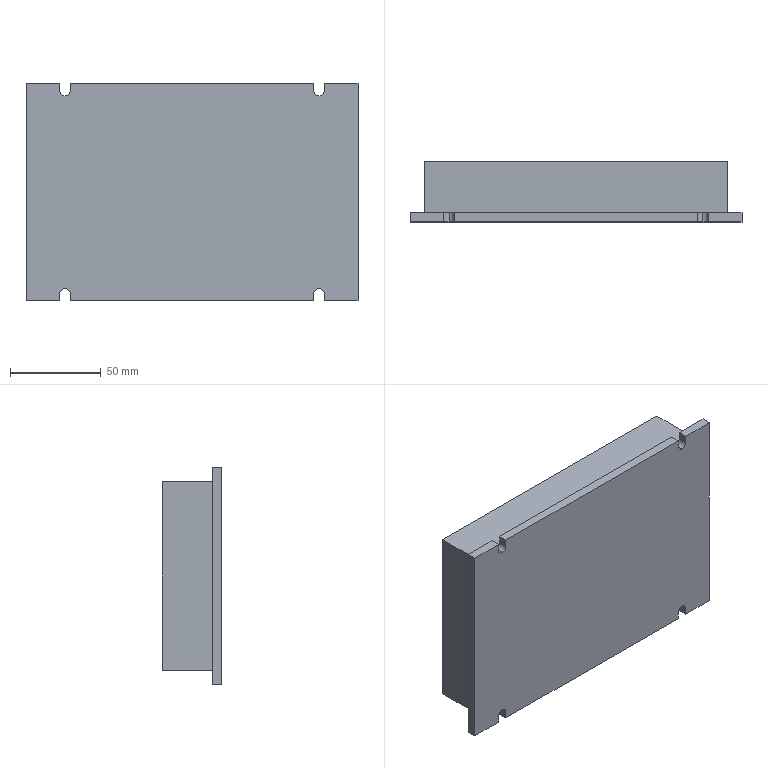Part | SolidWorks | features Extrusion 1, HoleWzd 1, ICE 1 | 1 solid | 29 faces | box 183 x 33 x 120 mm | volume 595376 mm3 | plane 23 | cylinder 6 | commonest cylinder face diameters 5.8 x6
STEP:
#1=CARTESIAN_POINT('',(-70.,5.,53.1));
#2=VERTEX_POINT('',#1);
#3=CARTESIAN_POINT('',(-67.1,5.,56.));
#4=VERTEX_POINT('',#3);
#5=CARTESIAN_POINT('',(-70.,5.,56.));
#6=DIRECTION('',(0.,-1.,0.));
#7=DIRECTION('',(0.,0.,-1.));
#8=AXIS2_PLACEMENT_3D('',#5,#6,#7);
#9=CIRCLE('',#8,2.9);
#10=EDGE_CURVE('',#2,#4,#9,.T.);
#11=ORIENTED_EDGE('',*,*,#10,.F.);
#12=CARTESIAN_POINT('',(-70.,0.,53.1));
#13=VERTEX_POINT('',#12);
#14=CARTESIAN_POINT('',(-70.,0.,53.1));
#15=DIRECTION('',(0.,-1.,0.));
#16=VECTOR('',#15,1000.);
#17=LINE('',#14,#16);
#18=EDGE_CURVE('',#2,#13,#17,.T.);
#19=ORIENTED_EDGE('',*,*,#18,.T.);
#20=CARTESIAN_POINT('',(-67.1,0.,56.));
#21=VERTEX_POINT('',#20);
#22=CARTESIAN_POINT('',(-70.,0.,56.));
#23=DIRECTION('',(0.,-1.,0.));
#24=DIRECTION('',(0.,0.,-1.));
#25=AXIS2_PLACEMENT_3D('',#22,#23,#24);
#26=CIRCLE('',#25,2.9);
#27=EDGE_CURVE('',#13,#21,#26,.T.);
#28=ORIENTED_EDGE('',*,*,#27,.T.);
#29=CARTESIAN_POINT('',(-67.1,33.,56.));
#30=DIRECTION('',(0.,1.,0.));
#31=VECTOR('',#30,1000.);
#32=LINE('',#29,#31);
#33=EDGE_CURVE('',#21,#4,#32,.T.);
#34=ORIENTED_EDGE('',*,*,#33,.T.);
#35=EDGE_LOOP('',(#11,#19,#28,#34));
#36=FACE_OUTER_BOUND('',#35,.T.);
#37=CARTESIAN_POINT('',(-70.,0.,56.));
#38=DIRECTION('',(0.,-1.,0.));
#39=DIRECTION('',(0.,0.,-1.));
#40=AXIS2_PLACEMENT_3D('',#37,#38,#39);
#41=CYLINDRICAL_SURFACE('',#40,2.9);
#42=ADVANCED_FACE('',(#36),#41,.F.);
#43=CARTESIAN_POINT('',(70.,5.,53.1));
#44=VERTEX_POINT('',#43);
#45=CARTESIAN_POINT('',(72.9,5.,56.));
#46=VERTEX_POINT('',#45);
#47=CARTESIAN_POINT('',(70.,5.,56.));
#48=DIRECTION('',(0.,-1.,0.));
#49=DIRECTION('',(0.,0.,-1.));
#50=AXIS2_PLACEMENT_3D('',#47,#48,#49);
#51=CIRCLE('',#50,2.9);
#52=EDGE_CURVE('',#44,#46,#51,.T.);
#53=ORIENTED_EDGE('',*,*,#52,.F.);
#54=CARTESIAN_POINT('',(70.,0.,53.1));
#55=VERTEX_POINT('',#54);
#56=CARTESIAN_POINT('',(70.,0.,53.1));
#57=DIRECTION('',(0.,-1.,0.));
#58=VECTOR('',#57,1000.);
#59=LINE('',#56,#58);
#60=EDGE_CURVE('',#44,#55,#59,.T.);
#61=ORIENTED_EDGE('',*,*,#60,.T.);
#62=CARTESIAN_POINT('',(72.9,0.,56.));
#63=VERTEX_POINT('',#62);
#64=CARTESIAN_POINT('',(70.,0.,56.));
#65=DIRECTION('',(0.,-1.,0.));
#66=DIRECTION('',(0.,0.,-1.));
#67=AXIS2_PLACEMENT_3D('',#64,#65,#66);
#68=CIRCLE('',#67,2.9);
#69=EDGE_CURVE('',#55,#63,#68,.T.);
#70=ORIENTED_EDGE('',*,*,#69,.T.);
#71=CARTESIAN_POINT('',(72.9,33.,56.));
#72=DIRECTION('',(0.,1.,0.));
#73=VECTOR('',#72,1000.);
#74=LINE('',#71,#73);
#75=EDGE_CURVE('',#63,#46,#74,.T.);
#76=ORIENTED_EDGE('',*,*,#75,.T.);
#77=EDGE_LOOP('',(#53,#61,#70,#76));
#78=FACE_OUTER_BOUND('',#77,.T.);
#79=CARTESIAN_POINT('',(70.,0.,56.));
#80=DIRECTION('',(0.,-1.,0.));
#81=DIRECTION('',(0.,0.,-1.));
#82=AXIS2_PLACEMENT_3D('',#79,#80,#81);
#83=CYLINDRICAL_SURFACE('',#82,2.9);
#84=ADVANCED_FACE('',(#78),#83,.F.);
#85=CARTESIAN_POINT('',(-83.5,5.,52.));
#86=VERTEX_POINT('',#85);
#87=CARTESIAN_POINT('',(83.5,5.,52.));
#88=VERTEX_POINT('',#87);
#89=CARTESIAN_POINT('',(-83.5,5.,52.));
#90=DIRECTION('',(1.,0.,0.));
#91=VECTOR('',#90,1000.);
#92=LINE('',#89,#91);
#93=EDGE_CURVE('',#86,#88,#92,.T.);
#94=ORIENTED_EDGE('',*,*,#93,.F.);
#95=CARTESIAN_POINT('',(-83.5,5.,-52.));
#96=VERTEX_POINT('',#95);
#97=CARTESIAN_POINT('',(-83.5,5.,-52.));
#98=DIRECTION('',(0.,0.,1.));
#99=VECTOR('',#98,1000.);
#100=LINE('',#97,#99);
#101=EDGE_CURVE('',#96,#86,#100,.T.);
#102=ORIENTED_EDGE('',*,*,#101,.F.);
#103=CARTESIAN_POINT('',(83.5,5.,-52.));
#104=VERTEX_POINT('',#103);
#105=CARTESIAN_POINT('',(83.5,5.,-52.));
#106=DIRECTION('',(-1.,0.,0.));
#107=VECTOR('',#106,1000.);
#108=LINE('',#105,#107);
#109=EDGE_CURVE('',#104,#96,#108,.T.);
#110=ORIENTED_EDGE('',*,*,#109,.F.);
#111=CARTESIAN_POINT('',(83.5,5.,52.));
#112=DIRECTION('',(0.,0.,-1.));
#113=VECTOR('',#112,1000.);
#114=LINE('',#111,#113);
#115=EDGE_CURVE('',#88,#104,#114,.T.);
#116=ORIENTED_EDGE('',*,*,#115,.F.);
#117=EDGE_LOOP('',(#94,#102,#110,#116));
#118=FACE_BOUND('',#117,.T.);
#119=CARTESIAN_POINT('',(72.9,5.,-56.));
#120=VERTEX_POINT('',#119);
#121=CARTESIAN_POINT('',(72.9,5.,-60.));
#122=VERTEX_POINT('',#121);
#123=CARTESIAN_POINT('',(72.9,5.,0.));
#124=DIRECTION('',(0.,0.,-1.));
#125=VECTOR('',#124,1000.);
#126=LINE('',#123,#125);
#127=EDGE_CURVE('',#120,#122,#126,.T.);
#128=ORIENTED_EDGE('',*,*,#127,.F.);
#129=CARTESIAN_POINT('',(67.1,5.,-56.));
#130=VERTEX_POINT('',#129);
#131=CARTESIAN_POINT('',(70.,5.,-56.));
#132=DIRECTION('',(0.,-1.,0.));
#133=DIRECTION('',(0.,0.,-1.));
#134=AXIS2_PLACEMENT_3D('',#131,#132,#133);
#135=CIRCLE('',#134,2.9);
#136=EDGE_CURVE('',#120,#130,#135,.T.);
#137=ORIENTED_EDGE('',*,*,#136,.T.);
#138=CARTESIAN_POINT('',(67.1,5.,-60.));
#139=VERTEX_POINT('',#138);
#140=CARTESIAN_POINT('',(67.1,5.,0.));
#141=DIRECTION('',(0.,0.,-1.));
#142=VECTOR('',#141,1000.);
#143=LINE('',#140,#142);
#144=EDGE_CURVE('',#130,#139,#143,.T.);
#145=ORIENTED_EDGE('',*,*,#144,.T.);
#146=CARTESIAN_POINT('',(-67.1,5.,-60.));
#147=VERTEX_POINT('',#146);
#148=CARTESIAN_POINT('',(-91.5,5.,-60.));
#149=DIRECTION('',(-1.,0.,0.));
#150=VECTOR('',#149,1000.);
#151=LINE('',#148,#150);
#152=EDGE_CURVE('',#139,#147,#151,.T.);
#153=ORIENTED_EDGE('',*,*,#152,.T.);
#154=CARTESIAN_POINT('',(-67.1,5.,-56.));
#155=VERTEX_POINT('',#154);
#156=CARTESIAN_POINT('',(-67.1,5.,0.));
#157=DIRECTION('',(0.,0.,-1.));
#158=VECTOR('',#157,1000.);
#159=LINE('',#156,#158);
#160=EDGE_CURVE('',#155,#147,#159,.T.);
#161=ORIENTED_EDGE('',*,*,#160,.F.);
#162=CARTESIAN_POINT('',(-72.9,5.,-56.));
#163=VERTEX_POINT('',#162);
#164=CARTESIAN_POINT('',(-70.,5.,-56.));
#165=DIRECTION('',(0.,-1.,0.));
#166=DIRECTION('',(0.,0.,-1.));
#167=AXIS2_PLACEMENT_3D('',#164,#165,#166);
#168=CIRCLE('',#167,2.9);
#169=EDGE_CURVE('',#155,#163,#168,.T.);
#170=ORIENTED_EDGE('',*,*,#169,.T.);
#171=CARTESIAN_POINT('',(-72.9,5.,-60.));
#172=VERTEX_POINT('',#171);
#173=CARTESIAN_POINT('',(-72.9,5.,0.));
#174=DIRECTION('',(0.,0.,-1.));
#175=VECTOR('',#174,1000.);
#176=LINE('',#173,#175);
#177=EDGE_CURVE('',#163,#172,#176,.T.);
#178=ORIENTED_EDGE('',*,*,#177,.T.);
#179=CARTESIAN_POINT('',(-91.5,5.,-60.));
#180=VERTEX_POINT('',#179);
#181=CARTESIAN_POINT('',(-91.5,5.,-60.));
#182=DIRECTION('',(-1.,0.,0.));
#183=VECTOR('',#182,1000.);
#184=LINE('',#181,#183);
#185=EDGE_CURVE('',#172,#180,#184,.T.);
#186=ORIENTED_EDGE('',*,*,#185,.T.);
#187=CARTESIAN_POINT('',(-91.5,5.,60.));
#188=VERTEX_POINT('',#187);
#189=CARTESIAN_POINT('',(-91.5,5.,60.));
#190=DIRECTION('',(0.,0.,1.));
#191=VECTOR('',#190,1000.);
#192=LINE('',#189,#191);
#193=EDGE_CURVE('',#180,#188,#192,.T.);
#194=ORIENTED_EDGE('',*,*,#193,.T.);
#195=CARTESIAN_POINT('',(-72.9,5.,60.));
#196=VERTEX_POINT('',#195);
#197=CARTESIAN_POINT('',(-91.5,5.,60.));
#198=DIRECTION('',(1.,0.,0.));
#199=VECTOR('',#198,1000.);
#200=LINE('',#197,#199);
#201=EDGE_CURVE('',#188,#196,#200,.T.);
#202=ORIENTED_EDGE('',*,*,#201,.T.);
#203=CARTESIAN_POINT('',(-72.9,5.,56.));
#204=VERTEX_POINT('',#203);
#205=CARTESIAN_POINT('',(-72.9,5.,0.));
#206=DIRECTION('',(0.,0.,-1.));
#207=VECTOR('',#206,1000.);
#208=LINE('',#205,#207);
#209=EDGE_CURVE('',#196,#204,#208,.T.);
#210=ORIENTED_EDGE('',*,*,#209,.T.);
#211=CARTESIAN_POINT('',(-70.,5.,56.));
#212=DIRECTION('',(0.,-1.,0.));
#213=DIRECTION('',(0.,0.,-1.));
#214=AXIS2_PLACEMENT_3D('',#211,#212,#213);
#215=CIRCLE('',#214,2.9);
#216=EDGE_CURVE('',#204,#2,#215,.T.);
#217=ORIENTED_EDGE('',*,*,#216,.T.);
#218=ORIENTED_EDGE('',*,*,#10,.T.);
#219=CARTESIAN_POINT('',(-67.1,5.,60.));
#220=VERTEX_POINT('',#219);
#221=CARTESIAN_POINT('',(-67.1,5.,0.));
#222=DIRECTION('',(0.,0.,-1.));
#223=VECTOR('',#222,1000.);
#224=LINE('',#221,#223);
#225=EDGE_CURVE('',#220,#4,#224,.T.);
#226=ORIENTED_EDGE('',*,*,#225,.F.);
#227=CARTESIAN_POINT('',(67.1,5.,60.));
#228=VERTEX_POINT('',#227);
#229=CARTESIAN_POINT('',(-91.5,5.,60.));
#230=DIRECTION('',(1.,0.,0.));
#231=VECTOR('',#230,1000.);
#232=LINE('',#229,#231);
#233=EDGE_CURVE('',#220,#228,#232,.T.);
#234=ORIENTED_EDGE('',*,*,#233,.T.);
#235=CARTESIAN_POINT('',(67.1,5.,56.));
#236=VERTEX_POINT('',#235);
#237=CARTESIAN_POINT('',(67.1,5.,0.));
#238=DIRECTION('',(0.,0.,-1.));
#239=VECTOR('',#238,1000.);
#240=LINE('',#237,#239);
#241=EDGE_CURVE('',#228,#236,#240,.T.);
#242=ORIENTED_EDGE('',*,*,#241,.T.);
#243=CARTESIAN_POINT('',(70.,5.,56.));
#244=DIRECTION('',(0.,-1.,0.));
#245=DIRECTION('',(0.,0.,-1.));
#246=AXIS2_PLACEMENT_3D('',#243,#244,#245);
#247=CIRCLE('',#246,2.9);
#248=EDGE_CURVE('',#236,#44,#247,.T.);
#249=ORIENTED_EDGE('',*,*,#248,.T.);
#250=ORIENTED_EDGE('',*,*,#52,.T.);
#251=CARTESIAN_POINT('',(72.9,5.,60.));
#252=VERTEX_POINT('',#251);
#253=CARTESIAN_POINT('',(72.9,5.,0.));
#254=DIRECTION('',(0.,0.,-1.));
#255=VECTOR('',#254,1000.);
#256=LINE('',#253,#255);
#257=EDGE_CURVE('',#252,#46,#256,.T.);
#258=ORIENTED_EDGE('',*,*,#257,.F.);
#259=CARTESIAN_POINT('',(91.5,5.,60.));
#260=VERTEX_POINT('',#259);
#261=CARTESIAN_POINT('',(-91.5,5.,60.));
#262=DIRECTION('',(1.,0.,0.));
#263=VECTOR('',#262,1000.);
#264=LINE('',#261,#263);
#265=EDGE_CURVE('',#252,#260,#264,.T.);
#266=ORIENTED_EDGE('',*,*,#265,.T.);
#267=CARTESIAN_POINT('',(91.5,5.,-60.));
#268=VERTEX_POINT('',#267);
#269=CARTESIAN_POINT('',(91.5,5.,60.));
#270=DIRECTION('',(0.,0.,-1.));
#271=VECTOR('',#270,1000.);
#272=LINE('',#269,#271);
#273=EDGE_CURVE('',#260,#268,#272,.T.);
#274=ORIENTED_EDGE('',*,*,#273,.T.);
#275=CARTESIAN_POINT('',(-91.5,5.,-60.));
#276=DIRECTION('',(-1.,0.,0.));
#277=VECTOR('',#276,1000.);
#278=LINE('',#275,#277);
#279=EDGE_CURVE('',#268,#122,#278,.T.);
#280=ORIENTED_EDGE('',*,*,#279,.T.);
#281=EDGE_LOOP('',(#128,#137,#145,#153,#161,#170,#178,#186,#194,#202,#210,#217,#218,#226,#234,#242,#249,#250,#258,#266,#274,#280));
#282=FACE_OUTER_BOUND('',#281,.T.);
#283=CARTESIAN_POINT('',(0.,5.,0.));
#284=DIRECTION('',(0.,-1.,0.));
#285=DIRECTION('',(0.,0.,-1.));
#286=AXIS2_PLACEMENT_3D('',#283,#284,#285);
#287=PLANE('',#286);
#288=ADVANCED_FACE('',(#118,#282),#287,.F.);
#289=CARTESIAN_POINT('',(72.9,0.,-60.));
#290=VERTEX_POINT('',#289);
#291=CARTESIAN_POINT('',(72.9,5.,-60.));
#292=DIRECTION('',(0.,-1.,0.));
#293=VECTOR('',#292,1000.);
#294=LINE('',#291,#293);
#295=EDGE_CURVE('',#122,#290,#294,.T.);
#296=ORIENTED_EDGE('',*,*,#295,.F.);
#297=ORIENTED_EDGE('',*,*,#279,.F.);
#298=CARTESIAN_POINT('',(91.5,0.,-60.));
#299=VERTEX_POINT('',#298);
#300=CARTESIAN_POINT('',(91.5,5.,-60.));
#301=DIRECTION('',(0.,-1.,0.));
#302=VECTOR('',#301,1000.);
#303=LINE('',#300,#302);
#304=EDGE_CURVE('',#268,#299,#303,.T.);
#305=ORIENTED_EDGE('',*,*,#304,.T.);
#306=CARTESIAN_POINT('',(-91.5,0.,-60.));
#307=DIRECTION('',(-1.,0.,0.));
#308=VECTOR('',#307,1000.);
#309=LINE('',#306,#308);
#310=EDGE_CURVE('',#299,#290,#309,.T.);
#311=ORIENTED_EDGE('',*,*,#310,.T.);
#312=EDGE_LOOP('',(#296,#297,#305,#311));
#313=FACE_OUTER_BOUND('',#312,.T.);
#314=CARTESIAN_POINT('',(-91.5,5.,-60.));
#315=DIRECTION('',(0.,0.,1.));
#316=DIRECTION('',(1.,0.,0.));
#317=AXIS2_PLACEMENT_3D('',#314,#315,#316);
#318=PLANE('',#317);
#319=ADVANCED_FACE('',(#313),#318,.F.);
#320=CARTESIAN_POINT('',(72.9,0.,-56.));
#321=VERTEX_POINT('',#320);
#322=CARTESIAN_POINT('',(67.1,0.,-56.));
#323=VERTEX_POINT('',#322);
#324=CARTESIAN_POINT('',(70.,0.,-56.));
#325=DIRECTION('',(0.,-1.,0.));
#326=DIRECTION('',(0.,0.,-1.));
#327=AXIS2_PLACEMENT_3D('',#324,#325,#326);
#328=CIRCLE('',#327,2.9);
#329=EDGE_CURVE('',#321,#323,#328,.T.);
#330=ORIENTED_EDGE('',*,*,#329,.F.);
#331=CARTESIAN_POINT('',(72.9,0.,-56.));
#332=DIRECTION('',(0.,0.,-1.));
#333=VECTOR('',#332,1000.);
#334=LINE('',#331,#333);
#335=EDGE_CURVE('',#321,#290,#334,.T.);
#336=ORIENTED_EDGE('',*,*,#335,.T.);
#337=ORIENTED_EDGE('',*,*,#310,.F.);
#338=CARTESIAN_POINT('',(91.5,0.,60.));
#339=VERTEX_POINT('',#338);
#340=CARTESIAN_POINT('',(91.5,0.,60.));
#341=DIRECTION('',(0.,0.,-1.));
#342=VECTOR('',#341,1000.);
#343=LINE('',#340,#342);
#344=EDGE_CURVE('',#339,#299,#343,.T.);
#345=ORIENTED_EDGE('',*,*,#344,.F.);
#346=CARTESIAN_POINT('',(72.9,0.,60.));
#347=VERTEX_POINT('',#346);
#348=CARTESIAN_POINT('',(-91.5,0.,60.));
#349=DIRECTION('',(1.,0.,0.));
#350=VECTOR('',#349,1000.);
#351=LINE('',#348,#350);
#352=EDGE_CURVE('',#347,#339,#351,.T.);
#353=ORIENTED_EDGE('',*,*,#352,.F.);
#354=CARTESIAN_POINT('',(72.9,0.,64.));
#355=DIRECTION('',(0.,0.,-1.));
#356=VECTOR('',#355,1000.);
#357=LINE('',#354,#356);
#358=EDGE_CURVE('',#347,#63,#357,.T.);
#359=ORIENTED_EDGE('',*,*,#358,.T.);
#360=ORIENTED_EDGE('',*,*,#69,.F.);
#361=CARTESIAN_POINT('',(67.1,0.,56.));
#362=VERTEX_POINT('',#361);
#363=CARTESIAN_POINT('',(70.,0.,56.));
#364=DIRECTION('',(0.,-1.,0.));
#365=DIRECTION('',(0.,0.,-1.));
#366=AXIS2_PLACEMENT_3D('',#363,#364,#365);
#367=CIRCLE('',#366,2.9);
#368=EDGE_CURVE('',#362,#55,#367,.T.);
#369=ORIENTED_EDGE('',*,*,#368,.F.);
#370=CARTESIAN_POINT('',(67.1,0.,60.));
#371=VERTEX_POINT('',#370);
#372=CARTESIAN_POINT('',(67.1,0.,0.));
#373=DIRECTION('',(0.,0.,-1.));
#374=VECTOR('',#373,1000.);
#375=LINE('',#372,#374);
#376=EDGE_CURVE('',#371,#362,#375,.T.);
#377=ORIENTED_EDGE('',*,*,#376,.F.);
#378=CARTESIAN_POINT('',(-67.1,0.,60.));
#379=VERTEX_POINT('',#378);
#380=CARTESIAN_POINT('',(-91.5,0.,60.));
#381=DIRECTION('',(1.,0.,0.));
#382=VECTOR('',#381,1000.);
#383=LINE('',#380,#382);
#384=EDGE_CURVE('',#379,#371,#383,.T.);
#385=ORIENTED_EDGE('',*,*,#384,.F.);
#386=CARTESIAN_POINT('',(-67.1,0.,64.));
#387=DIRECTION('',(0.,0.,-1.));
#388=VECTOR('',#387,1000.);
#389=LINE('',#386,#388);
#390=EDGE_CURVE('',#379,#21,#389,.T.);
#391=ORIENTED_EDGE('',*,*,#390,.T.);
#392=ORIENTED_EDGE('',*,*,#27,.F.);
#393=CARTESIAN_POINT('',(-72.9,0.,56.));
#394=VERTEX_POINT('',#393);
#395=CARTESIAN_POINT('',(-70.,0.,56.));
#396=DIRECTION('',(0.,-1.,0.));
#397=DIRECTION('',(0.,0.,-1.));
#398=AXIS2_PLACEMENT_3D('',#395,#396,#397);
#399=CIRCLE('',#398,2.9);
#400=EDGE_CURVE('',#394,#13,#399,.T.);
#401=ORIENTED_EDGE('',*,*,#400,.F.);
#402=CARTESIAN_POINT('',(-72.9,0.,60.));
#403=VERTEX_POINT('',#402);
#404=CARTESIAN_POINT('',(-72.9,0.,64.));
#405=DIRECTION('',(0.,0.,-1.));
#406=VECTOR('',#405,1000.);
#407=LINE('',#404,#406);
#408=EDGE_CURVE('',#403,#394,#407,.T.);
#409=ORIENTED_EDGE('',*,*,#408,.F.);
#410=CARTESIAN_POINT('',(-91.5,0.,60.));
#411=VERTEX_POINT('',#410);
#412=CARTESIAN_POINT('',(-91.5,0.,60.));
#413=DIRECTION('',(1.,0.,0.));
#414=VECTOR('',#413,1000.);
#415=LINE('',#412,#414);
#416=EDGE_CURVE('',#411,#403,#415,.T.);
#417=ORIENTED_EDGE('',*,*,#416,.F.);
#418=CARTESIAN_POINT('',(-91.5,0.,-60.));
#419=VERTEX_POINT('',#418);
#420=CARTESIAN_POINT('',(-91.5,0.,60.));
#421=DIRECTION('',(0.,0.,1.));
#422=VECTOR('',#421,1000.);
#423=LINE('',#420,#422);
#424=EDGE_CURVE('',#419,#411,#423,.T.);
#425=ORIENTED_EDGE('',*,*,#424,.F.);
#426=CARTESIAN_POINT('',(-72.9,0.,-60.));
#427=VERTEX_POINT('',#426);
#428=CARTESIAN_POINT('',(-91.5,0.,-60.));
#429=DIRECTION('',(-1.,0.,0.));
#430=VECTOR('',#429,1000.);
#431=LINE('',#428,#430);
#432=EDGE_CURVE('',#427,#419,#431,.T.);
#433=ORIENTED_EDGE('',*,*,#432,.F.);
#434=CARTESIAN_POINT('',(-72.9,0.,-56.));
#435=VERTEX_POINT('',#434);
#436=CARTESIAN_POINT('',(-72.9,0.,-56.));
#437=DIRECTION('',(0.,0.,-1.));
#438=VECTOR('',#437,1000.);
#439=LINE('',#436,#438);
#440=EDGE_CURVE('',#435,#427,#439,.T.);
#441=ORIENTED_EDGE('',*,*,#440,.F.);
#442=CARTESIAN_POINT('',(-67.1,0.,-56.));
#443=VERTEX_POINT('',#442);
#444=CARTESIAN_POINT('',(-70.,0.,-56.));
#445=DIRECTION('',(0.,-1.,0.));
#446=DIRECTION('',(0.,0.,-1.));
#447=AXIS2_PLACEMENT_3D('',#444,#445,#446);
#448=CIRCLE('',#447,2.9);
#449=EDGE_CURVE('',#443,#435,#448,.T.);
#450=ORIENTED_EDGE('',*,*,#449,.F.);
#451=CARTESIAN_POINT('',(-67.1,0.,-60.));
#452=VERTEX_POINT('',#451);
#453=CARTESIAN_POINT('',(-67.1,0.,-56.));
#454=DIRECTION('',(0.,0.,-1.));
#455=VECTOR('',#454,1000.);
#456=LINE('',#453,#455);
#457=EDGE_CURVE('',#443,#452,#456,.T.);
#458=ORIENTED_EDGE('',*,*,#457,.T.);
#459=CARTESIAN_POINT('',(67.1,0.,-60.));
#460=VERTEX_POINT('',#459);
#461=CARTESIAN_POINT('',(-91.5,0.,-60.));
#462=DIRECTION('',(-1.,0.,0.));
#463=VECTOR('',#462,1000.);
#464=LINE('',#461,#463);
#465=EDGE_CURVE('',#460,#452,#464,.T.);
#466=ORIENTED_EDGE('',*,*,#465,.F.);
#467=CARTESIAN_POINT('',(67.1,0.,-56.));
#468=DIRECTION('',(0.,0.,-1.));
#469=VECTOR('',#468,1000.);
#470=LINE('',#467,#469);
#471=EDGE_CURVE('',#323,#460,#470,.T.);
#472=ORIENTED_EDGE('',*,*,#471,.F.);
#473=EDGE_LOOP('',(#330,#336,#337,#345,#353,#359,#360,#369,#377,#385,#391,#392,#401,#409,#417,#425,#433,#441,#450,#458,#466,#472));
#474=FACE_OUTER_BOUND('',#473,.T.);
#475=CARTESIAN_POINT('',(0.,0.,0.));
#476=DIRECTION('',(0.,-1.,0.));
#477=DIRECTION('',(0.,0.,-1.));
#478=AXIS2_PLACEMENT_3D('',#475,#476,#477);
#479=PLANE('',#478);
#480=ADVANCED_FACE('',(#474),#479,.T.);
#481=ORIENTED_EDGE('',*,*,#152,.F.);
#482=CARTESIAN_POINT('',(67.1,5.,-60.));
#483=DIRECTION('',(0.,-1.,0.));
#484=VECTOR('',#483,1000.);
#485=LINE('',#482,#484);
#486=EDGE_CURVE('',#139,#460,#485,.T.);
#487=ORIENTED_EDGE('',*,*,#486,.T.);
#488=ORIENTED_EDGE('',*,*,#465,.T.);
#489=CARTESIAN_POINT('',(-67.1,5.,-60.));
#490=DIRECTION('',(0.,-1.,0.));
#491=VECTOR('',#490,1000.);
#492=LINE('',#489,#491);
#493=EDGE_CURVE('',#147,#452,#492,.T.);
#494=ORIENTED_EDGE('',*,*,#493,.F.);
#495=EDGE_LOOP('',(#481,#487,#488,#494));
#496=FACE_OUTER_BOUND('',#495,.T.);
#497=CARTESIAN_POINT('',(-91.5,5.,-60.));
#498=DIRECTION('',(0.,0.,1.));
#499=DIRECTION('',(1.,0.,0.));
#500=AXIS2_PLACEMENT_3D('',#497,#498,#499);
#501=PLANE('',#500);
#502=ADVANCED_FACE('',(#496),#501,.F.);
#503=CARTESIAN_POINT('',(-67.1,5.,60.));
#504=DIRECTION('',(0.,1.,0.));
#505=VECTOR('',#504,1000.);
#506=LINE('',#503,#505);
#507=EDGE_CURVE('',#379,#220,#506,.T.);
#508=ORIENTED_EDGE('',*,*,#507,.F.);
#509=ORIENTED_EDGE('',*,*,#384,.T.);
#510=CARTESIAN_POINT('',(67.1,5.,60.));
#511=DIRECTION('',(0.,1.,0.));
#512=VECTOR('',#511,1000.);
#513=LINE('',#510,#512);
#514=EDGE_CURVE('',#371,#228,#513,.T.);
#515=ORIENTED_EDGE('',*,*,#514,.T.);
#516=ORIENTED_EDGE('',*,*,#233,.F.);
#517=EDGE_LOOP('',(#508,#509,#515,#516));
#518=FACE_OUTER_BOUND('',#517,.T.);
#519=CARTESIAN_POINT('',(-91.5,5.,60.));
#520=DIRECTION('',(0.,0.,-1.));
#521=DIRECTION('',(-1.,0.,0.));
#522=AXIS2_PLACEMENT_3D('',#519,#520,#521);
#523=PLANE('',#522);
#524=ADVANCED_FACE('',(#518),#523,.F.);
#525=CARTESIAN_POINT('',(72.9,5.,60.));
#526=DIRECTION('',(0.,1.,0.));
#527=VECTOR('',#526,1000.);
#528=LINE('',#525,#527);
#529=EDGE_CURVE('',#347,#252,#528,.T.);
#530=ORIENTED_EDGE('',*,*,#529,.F.);
#531=ORIENTED_EDGE('',*,*,#352,.T.);
#532=CARTESIAN_POINT('',(91.5,5.,60.));
#533=DIRECTION('',(0.,-1.,0.));
#534=VECTOR('',#533,1000.);
#535=LINE('',#532,#534);
#536=EDGE_CURVE('',#260,#339,#535,.T.);
#537=ORIENTED_EDGE('',*,*,#536,.F.);
#538=ORIENTED_EDGE('',*,*,#265,.F.);
#539=EDGE_LOOP('',(#530,#531,#537,#538));
#540=FACE_OUTER_BOUND('',#539,.T.);
#541=CARTESIAN_POINT('',(-91.5,5.,60.));
#542=DIRECTION('',(0.,0.,-1.));
#543=DIRECTION('',(-1.,0.,0.));
#544=AXIS2_PLACEMENT_3D('',#541,#542,#543);
#545=PLANE('',#544);
#546=ADVANCED_FACE('',(#540),#545,.F.);
#547=ORIENTED_EDGE('',*,*,#344,.T.);
#548=ORIENTED_EDGE('',*,*,#304,.F.);
#549=ORIENTED_EDGE('',*,*,#273,.F.);
#550=ORIENTED_EDGE('',*,*,#536,.T.);
#551=EDGE_LOOP('',(#547,#548,#549,#550));
#552=FACE_OUTER_BOUND('',#551,.T.);
#553=CARTESIAN_POINT('',(91.5,5.,60.));
#554=DIRECTION('',(-1.,0.,0.));
#555=DIRECTION('',(0.,0.,1.));
#556=AXIS2_PLACEMENT_3D('',#553,#554,#555);
#557=PLANE('',#556);
#558=ADVANCED_FACE('',(#552),#557,.F.);
#559=ORIENTED_EDGE('',*,*,#185,.F.);
#560=CARTESIAN_POINT('',(-72.9,5.,-60.));
#561=DIRECTION('',(0.,-1.,0.));
#562=VECTOR('',#561,1000.);
#563=LINE('',#560,#562);
#564=EDGE_CURVE('',#172,#427,#563,.T.);
#565=ORIENTED_EDGE('',*,*,#564,.T.);
#566=ORIENTED_EDGE('',*,*,#432,.T.);
#567=CARTESIAN_POINT('',(-91.5,5.,-60.));
#568=DIRECTION('',(0.,-1.,0.));
#569=VECTOR('',#568,1000.);
#570=LINE('',#567,#569);
#571=EDGE_CURVE('',#180,#419,#570,.T.);
#572=ORIENTED_EDGE('',*,*,#571,.F.);
#573=EDGE_LOOP('',(#559,#565,#566,#572));
#574=FACE_OUTER_BOUND('',#573,.T.);
#575=CARTESIAN_POINT('',(-91.5,5.,-60.));
#576=DIRECTION('',(0.,0.,1.));
#577=DIRECTION('',(1.,0.,0.));
#578=AXIS2_PLACEMENT_3D('',#575,#576,#577);
#579=PLANE('',#578);
#580=ADVANCED_FACE('',(#574),#579,.F.);
#581=ORIENTED_EDGE('',*,*,#424,.T.);
#582=CARTESIAN_POINT('',(-91.5,5.,60.));
#583=DIRECTION('',(0.,-1.,0.));
#584=VECTOR('',#583,1000.);
#585=LINE('',#582,#584);
#586=EDGE_CURVE('',#188,#411,#585,.T.);
#587=ORIENTED_EDGE('',*,*,#586,.F.);
#588=ORIENTED_EDGE('',*,*,#193,.F.);
#589=ORIENTED_EDGE('',*,*,#571,.T.);
#590=EDGE_LOOP('',(#581,#587,#588,#589));
#591=FACE_OUTER_BOUND('',#590,.T.);
#592=CARTESIAN_POINT('',(-91.5,5.,60.));
#593=DIRECTION('',(1.,0.,0.));
#594=DIRECTION('',(0.,0.,-1.));
#595=AXIS2_PLACEMENT_3D('',#592,#593,#594);
#596=PLANE('',#595);
#597=ADVANCED_FACE('',(#591),#596,.F.);
#598=ORIENTED_EDGE('',*,*,#416,.T.);
#599=CARTESIAN_POINT('',(-72.9,5.,60.));
#600=DIRECTION('',(0.,1.,0.));
#601=VECTOR('',#600,1000.);
#602=LINE('',#599,#601);
#603=EDGE_CURVE('',#403,#196,#602,.T.);
#604=ORIENTED_EDGE('',*,*,#603,.T.);
#605=ORIENTED_EDGE('',*,*,#201,.F.);
#606=ORIENTED_EDGE('',*,*,#586,.T.);
#607=EDGE_LOOP('',(#598,#604,#605,#606));
#608=FACE_OUTER_BOUND('',#607,.T.);
#609=CARTESIAN_POINT('',(-91.5,5.,60.));
#610=DIRECTION('',(0.,0.,-1.));
#611=DIRECTION('',(-1.,0.,0.));
#612=AXIS2_PLACEMENT_3D('',#609,#610,#611);
#613=PLANE('',#612);
#614=ADVANCED_FACE('',(#608),#613,.F.);
#615=ORIENTED_EDGE('',*,*,#93,.T.);
#616=CARTESIAN_POINT('',(83.5,33.,52.));
#617=VERTEX_POINT('',#616);
#618=CARTESIAN_POINT('',(83.5,33.,52.));
#619=DIRECTION('',(0.,-1.,0.));
#620=VECTOR('',#619,1000.);
#621=LINE('',#618,#620);
#622=EDGE_CURVE('',#617,#88,#621,.T.);
#623=ORIENTED_EDGE('',*,*,#622,.F.);
#624=CARTESIAN_POINT('',(-83.5,33.,52.));
#625=VERTEX_POINT('',#624);
#626=CARTESIAN_POINT('',(-83.5,33.,52.));
#627=DIRECTION('',(1.,0.,0.));
#628=VECTOR('',#627,1000.);
#629=LINE('',#626,#628);
#630=EDGE_CURVE('',#625,#617,#629,.T.);
#631=ORIENTED_EDGE('',*,*,#630,.F.);
#632=CARTESIAN_POINT('',(-83.5,33.,52.));
#633=DIRECTION('',(0.,-1.,0.));
#634=VECTOR('',#633,1000.);
#635=LINE('',#632,#634);
#636=EDGE_CURVE('',#625,#86,#635,.T.);
#637=ORIENTED_EDGE('',*,*,#636,.T.);
#638=EDGE_LOOP('',(#615,#623,#631,#637));
#639=FACE_OUTER_BOUND('',#638,.T.);
#640=CARTESIAN_POINT('',(-83.5,33.,52.));
#641=DIRECTION('',(0.,0.,-1.));
#642=DIRECTION('',(-1.,0.,0.));
#643=AXIS2_PLACEMENT_3D('',#640,#641,#642);
#644=PLANE('',#643);
#645=ADVANCED_FACE('',(#639),#644,.F.);
#646=ORIENTED_EDGE('',*,*,#115,.T.);
#647=CARTESIAN_POINT('',(83.5,33.,-52.));
#648=VERTEX_POINT('',#647);
#649=CARTESIAN_POINT('',(83.5,33.,-52.));
#650=DIRECTION('',(0.,-1.,0.));
#651=VECTOR('',#650,1000.);
#652=LINE('',#649,#651);
#653=EDGE_CURVE('',#648,#104,#652,.T.);
#654=ORIENTED_EDGE('',*,*,#653,.F.);
#655=CARTESIAN_POINT('',(83.5,33.,52.));
#656=DIRECTION('',(0.,0.,-1.));
#657=VECTOR('',#656,1000.);
#658=LINE('',#655,#657);
#659=EDGE_CURVE('',#617,#648,#658,.T.);
#660=ORIENTED_EDGE('',*,*,#659,.F.);
#661=ORIENTED_EDGE('',*,*,#622,.T.);
#662=EDGE_LOOP('',(#646,#654,#660,#661));
#663=FACE_OUTER_BOUND('',#662,.T.);
#664=CARTESIAN_POINT('',(83.5,33.,52.));
#665=DIRECTION('',(-1.,0.,0.));
#666=DIRECTION('',(0.,0.,1.));
#667=AXIS2_PLACEMENT_3D('',#664,#665,#666);
#668=PLANE('',#667);
#669=ADVANCED_FACE('',(#663),#668,.F.);
#670=ORIENTED_EDGE('',*,*,#109,.T.);
#671=CARTESIAN_POINT('',(-83.5,33.,-52.));
#672=VERTEX_POINT('',#671);
#673=CARTESIAN_POINT('',(-83.5,33.,-52.));
#674=DIRECTION('',(0.,-1.,0.));
#675=VECTOR('',#674,1000.);
#676=LINE('',#673,#675);
#677=EDGE_CURVE('',#672,#96,#676,.T.);
#678=ORIENTED_EDGE('',*,*,#677,.F.);
#679=CARTESIAN_POINT('',(83.5,33.,-52.));
#680=DIRECTION('',(-1.,0.,0.));
#681=VECTOR('',#680,1000.);
#682=LINE('',#679,#681);
#683=EDGE_CURVE('',#648,#672,#682,.T.);
#684=ORIENTED_EDGE('',*,*,#683,.F.);
#685=ORIENTED_EDGE('',*,*,#653,.T.);
#686=EDGE_LOOP('',(#670,#678,#684,#685));
#687=FACE_OUTER_BOUND('',#686,.T.);
#688=CARTESIAN_POINT('',(83.5,33.,-52.));
#689=DIRECTION('',(0.,0.,1.));
#690=DIRECTION('',(1.,0.,0.));
#691=AXIS2_PLACEMENT_3D('',#688,#689,#690);
#692=PLANE('',#691);
#693=ADVANCED_FACE('',(#687),#692,.F.);
#694=ORIENTED_EDGE('',*,*,#101,.T.);
#695=ORIENTED_EDGE('',*,*,#636,.F.);
#696=CARTESIAN_POINT('',(-83.5,33.,-52.));
#697=DIRECTION('',(0.,0.,1.));
#698=VECTOR('',#697,1000.);
#699=LINE('',#696,#698);
#700=EDGE_CURVE('',#672,#625,#699,.T.);
#701=ORIENTED_EDGE('',*,*,#700,.F.);
#702=ORIENTED_EDGE('',*,*,#677,.T.);
#703=EDGE_LOOP('',(#694,#695,#701,#702));
#704=FACE_OUTER_BOUND('',#703,.T.);
#705=CARTESIAN_POINT('',(-83.5,33.,-52.));
#706=DIRECTION('',(1.,0.,0.));
#707=DIRECTION('',(0.,0.,-1.));
#708=AXIS2_PLACEMENT_3D('',#705,#706,#707);
#709=PLANE('',#708);
#710=ADVANCED_FACE('',(#704),#709,.F.);
#711=ORIENTED_EDGE('',*,*,#630,.T.);
#712=ORIENTED_EDGE('',*,*,#659,.T.);
#713=ORIENTED_EDGE('',*,*,#683,.T.);
#714=ORIENTED_EDGE('',*,*,#700,.T.);
#715=EDGE_LOOP('',(#711,#712,#713,#714));
#716=FACE_OUTER_BOUND('',#715,.T.);
#717=CARTESIAN_POINT('',(0.,33.,0.));
#718=DIRECTION('',(0.,1.,0.));
#719=DIRECTION('',(0.,0.,1.));
#720=AXIS2_PLACEMENT_3D('',#717,#718,#719);
#721=PLANE('',#720);
#722=ADVANCED_FACE('',(#716),#721,.T.);
#723=ORIENTED_EDGE('',*,*,#60,.F.);
#724=ORIENTED_EDGE('',*,*,#248,.F.);
#725=CARTESIAN_POINT('',(67.1,0.,56.));
#726=DIRECTION('',(0.,1.,0.));
#727=VECTOR('',#726,1000.);
#728=LINE('',#725,#727);
#729=EDGE_CURVE('',#362,#236,#728,.T.);
#730=ORIENTED_EDGE('',*,*,#729,.F.);
#731=ORIENTED_EDGE('',*,*,#368,.T.);
#732=EDGE_LOOP('',(#723,#724,#730,#731));
#733=FACE_OUTER_BOUND('',#732,.T.);
#734=CARTESIAN_POINT('',(70.,0.,56.));
#735=DIRECTION('',(0.,-1.,0.));
#736=DIRECTION('',(0.,0.,-1.));
#737=AXIS2_PLACEMENT_3D('',#734,#735,#736);
#738=CYLINDRICAL_SURFACE('',#737,2.9);
#739=ADVANCED_FACE('',(#733),#738,.F.);
#740=ORIENTED_EDGE('',*,*,#257,.T.);
#741=ORIENTED_EDGE('',*,*,#75,.F.);
#742=ORIENTED_EDGE('',*,*,#358,.F.);
#743=ORIENTED_EDGE('',*,*,#529,.T.);
#744=EDGE_LOOP('',(#740,#741,#742,#743));
#745=FACE_OUTER_BOUND('',#744,.T.);
#746=CARTESIAN_POINT('',(72.9,33.,64.));
#747=DIRECTION('',(-1.,0.,0.));
#748=DIRECTION('',(0.,-1.,0.));
#749=AXIS2_PLACEMENT_3D('',#746,#747,#748);
#750=PLANE('',#749);
#751=ADVANCED_FACE('',(#745),#750,.T.);
#752=ORIENTED_EDGE('',*,*,#514,.F.);
#753=ORIENTED_EDGE('',*,*,#376,.T.);
#754=ORIENTED_EDGE('',*,*,#729,.T.);
#755=ORIENTED_EDGE('',*,*,#241,.F.);
#756=EDGE_LOOP('',(#752,#753,#754,#755));
#757=FACE_OUTER_BOUND('',#756,.T.);
#758=CARTESIAN_POINT('',(67.1,0.,64.));
#759=DIRECTION('',(-1.,0.,0.));
#760=DIRECTION('',(0.,0.,1.));
#761=AXIS2_PLACEMENT_3D('',#758,#759,#760);
#762=PLANE('',#761);
#763=ADVANCED_FACE('',(#757),#762,.F.);
#764=ORIENTED_EDGE('',*,*,#18,.F.);
#765=ORIENTED_EDGE('',*,*,#216,.F.);
#766=CARTESIAN_POINT('',(-72.9,0.,56.));
#767=DIRECTION('',(0.,1.,0.));
#768=VECTOR('',#767,1000.);
#769=LINE('',#766,#768);
#770=EDGE_CURVE('',#394,#204,#769,.T.);
#771=ORIENTED_EDGE('',*,*,#770,.F.);
#772=ORIENTED_EDGE('',*,*,#400,.T.);
#773=EDGE_LOOP('',(#764,#765,#771,#772));
#774=FACE_OUTER_BOUND('',#773,.T.);
#775=CARTESIAN_POINT('',(-70.,0.,56.));
#776=DIRECTION('',(0.,-1.,0.));
#777=DIRECTION('',(0.,0.,-1.));
#778=AXIS2_PLACEMENT_3D('',#775,#776,#777);
#779=CYLINDRICAL_SURFACE('',#778,2.9);
#780=ADVANCED_FACE('',(#774),#779,.F.);
#781=ORIENTED_EDGE('',*,*,#225,.T.);
#782=ORIENTED_EDGE('',*,*,#33,.F.);
#783=ORIENTED_EDGE('',*,*,#390,.F.);
#784=ORIENTED_EDGE('',*,*,#507,.T.);
#785=EDGE_LOOP('',(#781,#782,#783,#784));
#786=FACE_OUTER_BOUND('',#785,.T.);
#787=CARTESIAN_POINT('',(-67.1,33.,64.));
#788=DIRECTION('',(-1.,0.,0.));
#789=DIRECTION('',(0.,-1.,0.));
#790=AXIS2_PLACEMENT_3D('',#787,#788,#789);
#791=PLANE('',#790);
#792=ADVANCED_FACE('',(#786),#791,.T.);
#793=ORIENTED_EDGE('',*,*,#603,.F.);
#794=ORIENTED_EDGE('',*,*,#408,.T.);
#795=ORIENTED_EDGE('',*,*,#770,.T.);
#796=ORIENTED_EDGE('',*,*,#209,.F.);
#797=EDGE_LOOP('',(#793,#794,#795,#796));
#798=FACE_OUTER_BOUND('',#797,.T.);
#799=CARTESIAN_POINT('',(-72.9,0.,64.));
#800=DIRECTION('',(-1.,0.,0.));
#801=DIRECTION('',(0.,0.,1.));
#802=AXIS2_PLACEMENT_3D('',#799,#800,#801);
#803=PLANE('',#802);
#804=ADVANCED_FACE('',(#798),#803,.F.);
#805=ORIENTED_EDGE('',*,*,#160,.T.);
#806=ORIENTED_EDGE('',*,*,#493,.T.);
#807=ORIENTED_EDGE('',*,*,#457,.F.);
#808=CARTESIAN_POINT('',(-67.1,33.,-56.));
#809=DIRECTION('',(0.,1.,0.));
#810=VECTOR('',#809,1000.);
#811=LINE('',#808,#810);
#812=EDGE_CURVE('',#443,#155,#811,.T.);
#813=ORIENTED_EDGE('',*,*,#812,.T.);
#814=EDGE_LOOP('',(#805,#806,#807,#813));
#815=FACE_OUTER_BOUND('',#814,.T.);
#816=CARTESIAN_POINT('',(-67.1,33.,-56.));
#817=DIRECTION('',(-1.,0.,0.));
#818=DIRECTION('',(0.,-1.,0.));
#819=AXIS2_PLACEMENT_3D('',#816,#817,#818);
#820=PLANE('',#819);
#821=ADVANCED_FACE('',(#815),#820,.T.);
#822=CARTESIAN_POINT('',(-72.9,0.,-56.));
#823=DIRECTION('',(0.,-1.,0.));
#824=VECTOR('',#823,1000.);
#825=LINE('',#822,#824);
#826=EDGE_CURVE('',#163,#435,#825,.T.);
#827=ORIENTED_EDGE('',*,*,#826,.T.);
#828=ORIENTED_EDGE('',*,*,#440,.T.);
#829=ORIENTED_EDGE('',*,*,#564,.F.);
#830=ORIENTED_EDGE('',*,*,#177,.F.);
#831=EDGE_LOOP('',(#827,#828,#829,#830));
#832=FACE_OUTER_BOUND('',#831,.T.);
#833=CARTESIAN_POINT('',(-72.9,0.,-56.));
#834=DIRECTION('',(-1.,0.,0.));
#835=DIRECTION('',(0.,0.,1.));
#836=AXIS2_PLACEMENT_3D('',#833,#834,#835);
#837=PLANE('',#836);
#838=ADVANCED_FACE('',(#832),#837,.F.);
#839=ORIENTED_EDGE('',*,*,#812,.F.);
#840=ORIENTED_EDGE('',*,*,#449,.T.);
#841=ORIENTED_EDGE('',*,*,#826,.F.);
#842=ORIENTED_EDGE('',*,*,#169,.F.);
#843=EDGE_LOOP('',(#839,#840,#841,#842));
#844=FACE_OUTER_BOUND('',#843,.T.);
#845=CARTESIAN_POINT('',(-70.,0.,-56.));
#846=DIRECTION('',(0.,-1.,0.));
#847=DIRECTION('',(0.,0.,-1.));
#848=AXIS2_PLACEMENT_3D('',#845,#846,#847);
#849=CYLINDRICAL_SURFACE('',#848,2.9);
#850=ADVANCED_FACE('',(#844),#849,.F.);
#851=ORIENTED_EDGE('',*,*,#127,.T.);
#852=ORIENTED_EDGE('',*,*,#295,.T.);
#853=ORIENTED_EDGE('',*,*,#335,.F.);
#854=CARTESIAN_POINT('',(72.9,33.,-56.));
#855=DIRECTION('',(0.,1.,0.));
#856=VECTOR('',#855,1000.);
#857=LINE('',#854,#856);
#858=EDGE_CURVE('',#321,#120,#857,.T.);
#859=ORIENTED_EDGE('',*,*,#858,.T.);
#860=EDGE_LOOP('',(#851,#852,#853,#859));
#861=FACE_OUTER_BOUND('',#860,.T.);
#862=CARTESIAN_POINT('',(72.9,33.,-56.));
#863=DIRECTION('',(-1.,0.,0.));
#864=DIRECTION('',(0.,-1.,0.));
#865=AXIS2_PLACEMENT_3D('',#862,#863,#864);
#866=PLANE('',#865);
#867=ADVANCED_FACE('',(#861),#866,.T.);
#868=CARTESIAN_POINT('',(67.1,0.,-56.));
#869=DIRECTION('',(0.,-1.,0.));
#870=VECTOR('',#869,1000.);
#871=LINE('',#868,#870);
#872=EDGE_CURVE('',#130,#323,#871,.T.);
#873=ORIENTED_EDGE('',*,*,#872,.T.);
#874=ORIENTED_EDGE('',*,*,#471,.T.);
#875=ORIENTED_EDGE('',*,*,#486,.F.);
#876=ORIENTED_EDGE('',*,*,#144,.F.);
#877=EDGE_LOOP('',(#873,#874,#875,#876));
#878=FACE_OUTER_BOUND('',#877,.T.);
#879=CARTESIAN_POINT('',(67.1,0.,-56.));
#880=DIRECTION('',(-1.,0.,0.));
#881=DIRECTION('',(0.,0.,1.));
#882=AXIS2_PLACEMENT_3D('',#879,#880,#881);
#883=PLANE('',#882);
#884=ADVANCED_FACE('',(#878),#883,.F.);
#885=ORIENTED_EDGE('',*,*,#858,.F.);
#886=ORIENTED_EDGE('',*,*,#329,.T.);
#887=ORIENTED_EDGE('',*,*,#872,.F.);
#888=ORIENTED_EDGE('',*,*,#136,.F.);
#889=EDGE_LOOP('',(#885,#886,#887,#888));
#890=FACE_OUTER_BOUND('',#889,.T.);
#891=CARTESIAN_POINT('',(70.,0.,-56.));
#892=DIRECTION('',(0.,-1.,0.));
#893=DIRECTION('',(0.,0.,-1.));
#894=AXIS2_PLACEMENT_3D('',#891,#892,#893);
#895=CYLINDRICAL_SURFACE('',#894,2.9);
#896=ADVANCED_FACE('',(#890),#895,.F.);
#897=CLOSED_SHELL('',(#42,#84,#288,#319,#480,#502,#524,#546,#558,#580,#597,#614,#645,#669,#693,#710,#722,#739,#751,#763,#780,#792,#804,#821,#838,#850,#867,#884,#896));
#898=MANIFOLD_SOLID_BREP('',#897);
#899=CARTESIAN_POINT('',(0.,0.,0.));
#900=DIRECTION('',(0.,0.,1.));
#901=DIRECTION('',(1.,0.,0.));
#902=AXIS2_PLACEMENT_3D('',#899,#900,#901);
#903=(LENGTH_UNIT()NAMED_UNIT(*)SI_UNIT(.MILLI.,.METRE.));
#904=UNCERTAINTY_MEASURE_WITH_UNIT(LENGTH_MEASURE(0.00001),#903,'','');
#905=(NAMED_UNIT(*)PLANE_ANGLE_UNIT()SI_UNIT($,.RADIAN.));
#906=(NAMED_UNIT(*)SI_UNIT($,.STERADIAN.)SOLID_ANGLE_UNIT());
#907=(GEOMETRIC_REPRESENTATION_CONTEXT(3)GLOBAL_UNCERTAINTY_ASSIGNED_CONTEXT((#904))GLOBAL_UNIT_ASSIGNED_CONTEXT((#903,#905,#906))REPRESENTATION_CONTEXT('',''));
#908=ADVANCED_BREP_SHAPE_REPRESENTATION('',(#898,#902),#907);